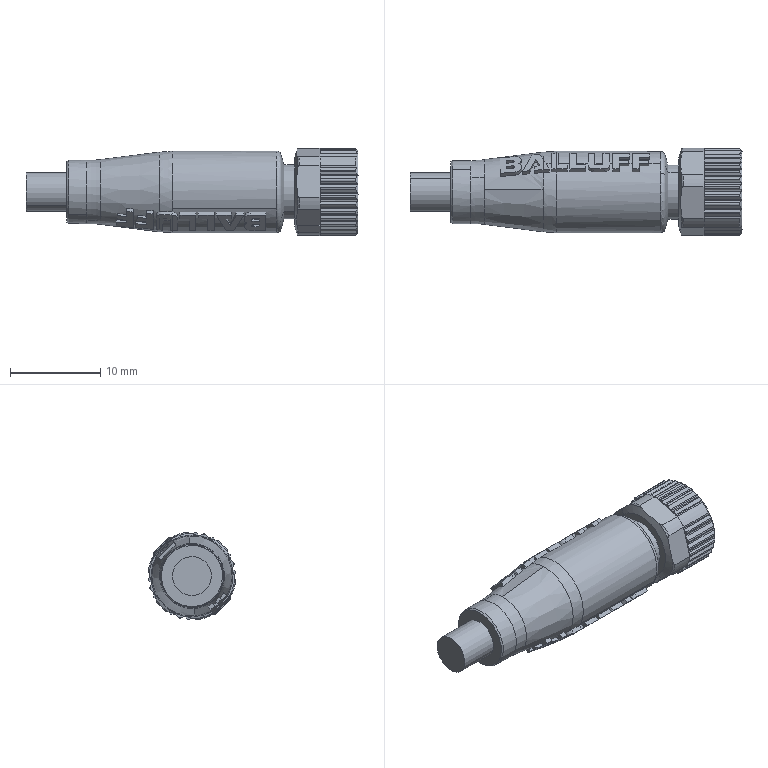Part | 1 solid | 419 faces | box 36.7 x 9.656 x 9.656 mm | volume 1818 mm3 | plane 248 | cylinder 132 | cone 26 | torus 10 | spline 3 | commonest cylinder face diameters 0.3 x54 1.05 x6 9.7 x6 9 x5 0.4 x4 1.181 x4